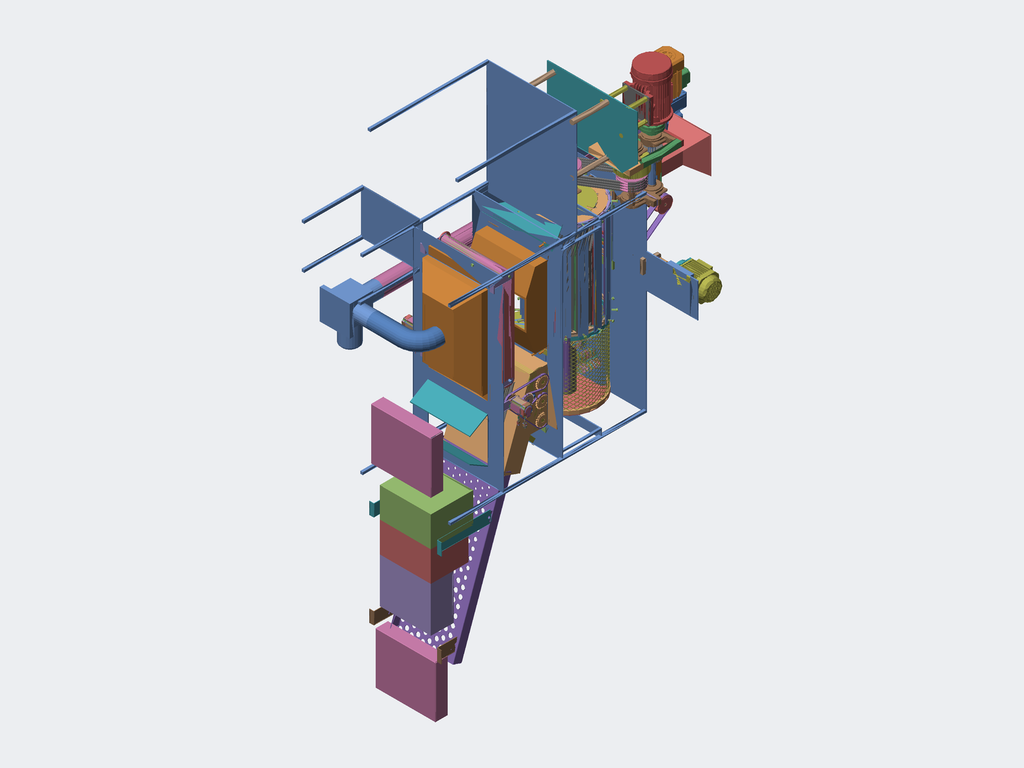Assembly | SolidWorks | 108 different items | 293 placed
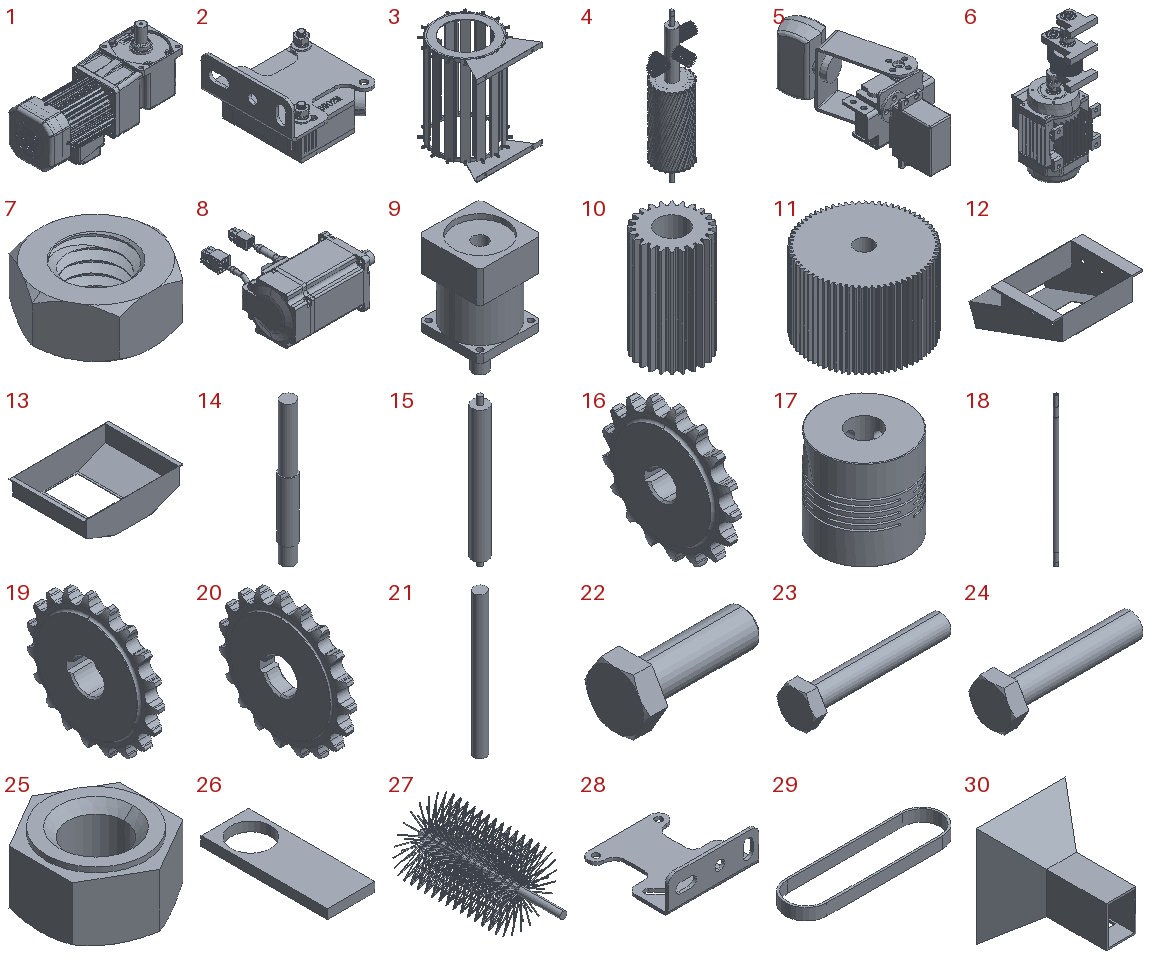Parts list (item | name | quantity | parent item | size | volume | features):
1 | (subassembly) | x1 | - | - | 5746372 mm3 | -
2 | (subassembly) | x1 | - | 60 x 58 x 40 mm | 49039 mm3 | features CompositeCurve 4
3 | (subassembly) | x1 | - | 488.345 x 547.074 x 650 mm | 5070939 mm3 | features ReferencePattern 72, LocalCirPattern 2, MirrorCompFeat 1
4 | (subassembly) | x1 | - | - | 9398103 mm3 | features ReferencePattern 46, LocalCirPattern 2
5 | (subassembly) | x1 | - | 62.179 x 144.352 x 61.763 mm | 114357 mm3 | features MirrorCompFeat 1
6 | (subassembly) | x1 | - | 154 x 213.028 x 468.972 mm | 4044827 mm3 | features AEMSimFeature 1
7 | - | x2 | in 2 | 7.91 x 6.85 x 3.05 mm | 87.239 mm3 | features Chamfer 1, Extrusion 1, Helix 1, ICE 1, RevCut 1, SweepCut 1
8 | - | x2 | - | - | - | features RefSurface 10
9 | - | x1 | - | 60 x 60 x 113 mm | 251469 mm3 | features ICE 7, Extrusion 1, RefAxis 1, RevCut 1
10 | - | x1 | in 6 | 26 x 26 x 44 mm | 14300 mm3 | features BaseBody 1, ICE 1
11 | - | x1 | in 6 | 71.959 x 72 x 50 mm | 185483 mm3 | features ICE 2, BaseBody 1
12 | - | x1 | - | 520 x 538.979 x 311.271 mm | 1451807 mm3 | features ICE 4, Extrusion 1, Shell 1
13 | - | x1 | - | 540 x 400 x 150 mm | 765108 mm3 | features ICE 3, Extrusion 1, Shell 1
14 | - | x1 | - | 40 x 40 x 355 mm | 385729 mm3 | features ICE 2, Extrusion 1
15 | - | x1 | - | 50 x 50 x 470 mm | 833504 mm3 | features ICE 2, Extrusion 1
16 | - | x2 | - | 15 x 73.539 x 73.841 mm | 33361 mm3 | features Chamfer 2, Cut 2, Revolution 2, CirPattern 1
17 | - | x2 | in 6 | 34 x 34 x 35 mm | 24409 mm3 | features BaseBody 1
18 | - | x2 | in 4 | 40 x 40 x 1400 mm | 1632189 mm3 | features ICE 6, Chamfer 4, 3DProfileFeature 1, Extrusion 1, HoleWzd 1, MoveCopyBody 1
19 | - | x3 | - | 15 x 81.595 x 81.862 mm | 41818 mm3 | features Chamfer 2, Cut 2, Revolution 2, CirPattern 1
20 | - | x1 | - | 9.37 x 81.595 x 81.862 mm | 34307 mm3 | features Chamfer 3, Cut 2, Revolution 2, CirPattern 1
21 | - | x1 | - | 30 x 30 x 352 mm | 248814 mm3 | features Extrusion 1, ICE 1
22 | - | x13 | - | 36.4 x 18.475 x 16 mm | 3737 mm3 | features BaseBody 1, Chamfer 1, ICE 1
23 | - | x48 | in 4 | 55.3 x 15.011 x 13 mm | 3267 mm3 | features BaseBody 1, MoveFace 1
24 | - | x30 | in 3 | 45.3 x 15.011 x 13 mm | 2757 mm3 | features BaseBody 1, RefAxis 1
25 | - | x1 | - | 13 x 15.011 x 7.5 mm | 785.095 mm3 | features BaseBody 1
26 | - | x1 | - | 60 x 160 x 12 mm | 91638 mm3 | features Extrusion 1, ICE 1
27 | - | x4 | in 4 | 100 x 200 x 100 mm | 28903 mm3 | features CirPattern 1, Extrusion 1, ICE 1, LPattern 1, RefAxis 1
28 | - | x1 | in 2 | 58 x 60 x 22 mm | 6510 mm3 | features ICE 3, MirrorPattern 2, SketchHole 2, EdgeFlange 1, Fillet 1, FlatPattern 1, SMBaseFlange 1, SheetMetal 1
29 | - | x1 | - | 378 x 100 x 28 mm | 119623 mm3 | features Extrusion 1
30 | - | x1 | - | 240 x 270 x 270 mm | 740709 mm3 | features ICE 3, Blend 1, Extrusion 1, Shell 1
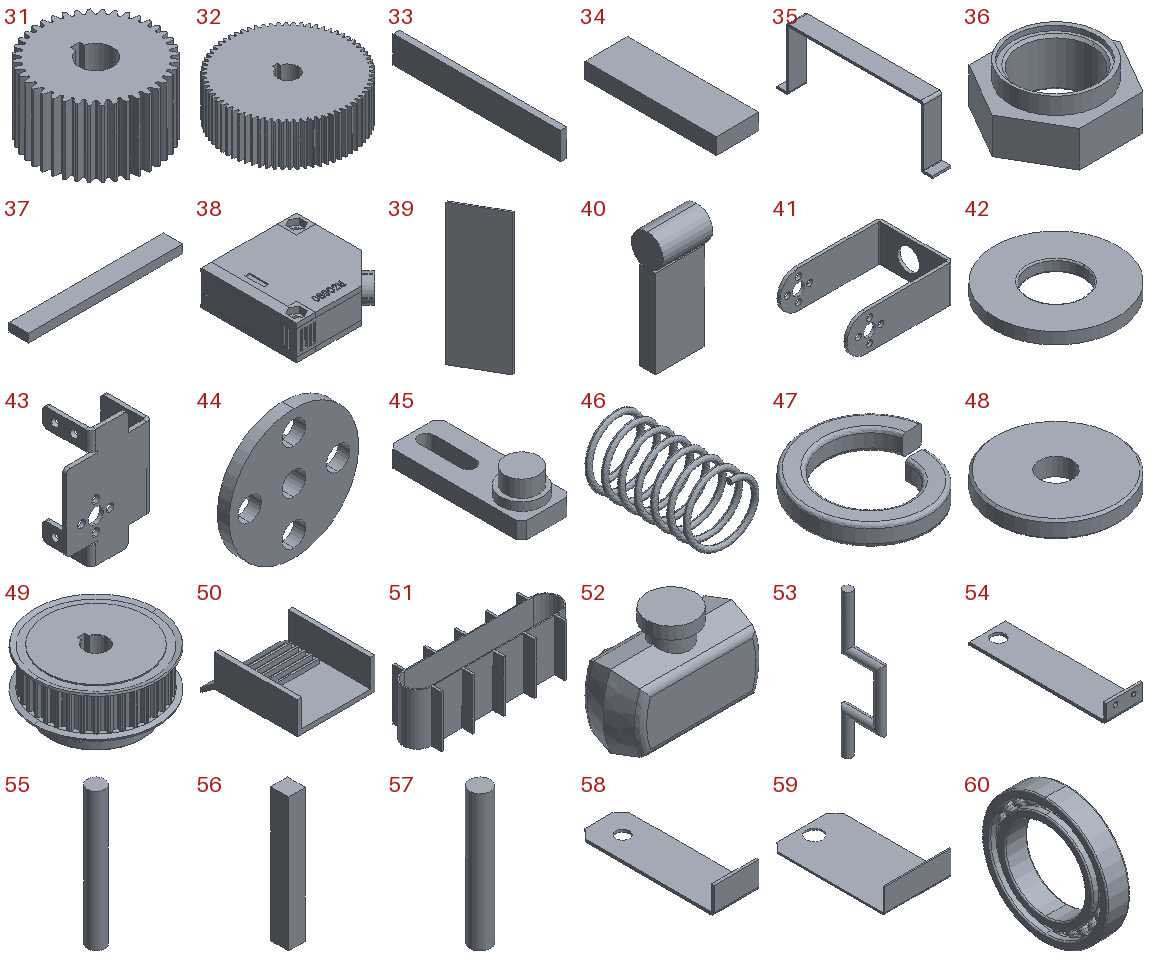31 | - | x1 | - | 104.808 x 104.808 x 60 mm | 422775 mm3 | features ICE 3, CirPattern 1, Extrusion 1, RefAxis 1
32 | - | x1 | - | 180 x 179.897 x 60 mm | 1397109 mm3 | features ICE 3, CirPattern 1, Extrusion 1, RefAxis 1
33 | - | x1 | - | 8 x 210 x 34 mm | 57120 mm3 | features Extrusion 1
34 | - | x1 | - | 90 x 275 x 34 mm | 841500 mm3 | features Extrusion 1
35 | - | x1 | - | 40 x 340 x 135 mm | 118889 mm3 | features EdgeFlange 2, FlatPattern 1, SMBaseFlange 1, SheetMetal 1
36 | - | x1 | - | 53.116 x 46 x 22 mm | 19269 mm3 | features ICE 3, Chamfer 1, Extrusion 1
37 | - | x1 | - | 275 x 34 x 15 mm | 140250 mm3 | features Extrusion 1
38 | - | x1 | in 2 | 50 x 50 x 18 mm | 41624 mm3 | features ICE 29, LPattern 4, CirPattern 2, Fillet 2, Chamfer 1, Extrusion 1, MirrorPattern 1
39 | - | x2 | - | 74.282 x 120 x 400 mm | 240000 mm3 | features Extrusion 1
40 | - | x1 | - | 62 x 50 x 150 mm | 220595 mm3 | features ICE 2, Extrusion 1
41 | - | x1 | in 5 | 71.712 x 49.895 x 25 mm | 8226 mm3 | features ICE 3, FlatPattern 1, SM3dBend 1, SMBaseFlange 1, SheetMetal 1
42 | - | x2 | in 2 | 9.05 x 9.05 x 0.85 mm | 43.941 mm3 | features Extrusion 1, Fillet 1, ICE 1
43 | - | x1 | in 5 | 45 x 25 x 62 mm | 6846 mm3 | features ICE 5, Fillet 3, EdgeFlange 2, SMBaseFlange 2, FlatPattern 1, MirrorPattern 1, SheetMetal 1
44 | - | x2 | in 5 | 22 x 6 x 22 mm | 838.805 mm3 | features ICE 2, Extrusion 1
45 | - | x1 | - | 30 x 80 x 25 mm | 26530 mm3 | features ICE 3, Chamfer 1, Extrusion 1
46 | - | x30 | in 3 | 12 x 23.5 x 12 mm | 203.726 mm3 | features Helix 1, Sweep 1
47 | - | x2 | in 2 | 6.6 x 6.6 x 2.189 mm | 20.119 mm3 | features Helix 1, Sweep 1
48 | - | x1 | - | 56 x 56 x 8 mm | 18117 mm3 | features Chamfer 1, Extrusion 1
49 | - | x2 | - | 99 x 99 x 48.077 mm | 252335 mm3 | features BaseBody 1
50 | - | x1 | - | 170 x 210 x 91.006 mm | 600000 mm3 | features ICE 3, Extrusion 1, LPattern 1
51 | - | x1 | - | 304 x 94 x 100 mm | 212673 mm3 | features ICE 2, LPattern 2, Extrusion 1
52 | - | x1 | in 5 | - | - | features ICE 4, Fillet 3, Extrusion 1, RevolvRefSurf 1
53 | - | x1 | - | 14 x 64 x 220 mm | 49260 mm3 | features Sweep 1
54 | - | x4 | - | 40 x 150 x 20 mm | 19277 mm3 | features ICE 2, EdgeFlange 1, FlatPattern 1, SMBaseFlange 1, SheetMetal 1
55 | - | x4 | - | 30 x 30 x 236 mm | 166819 mm3 | features Extrusion 1
56 | - | x2 | - | 32 x 34 x 253 mm | 275264 mm3 | features Extrusion 1
57 | - | x4 | - | 25 x 25 x 165 mm | 80994 mm3 | features Extrusion 1
58 | - | x5 | - | 50 x 154 x 30 mm | 26176 mm3 | features Chamfer 1, EdgeFlange 1, FlatPattern 1, ICE 1, SMBaseFlange 1, SheetMetal 1
59 | - | x2 | - | 80 x 140 x 30 mm | 25932 mm3 | features Chamfer 1, EdgeFlange 1, FlatPattern 1, ICE 1, SMBaseFlange 1, SheetMetal 1
60 | - | x2 | - | 10 x 55 x 55 mm | 10471 mm3 | features BaseBody 25
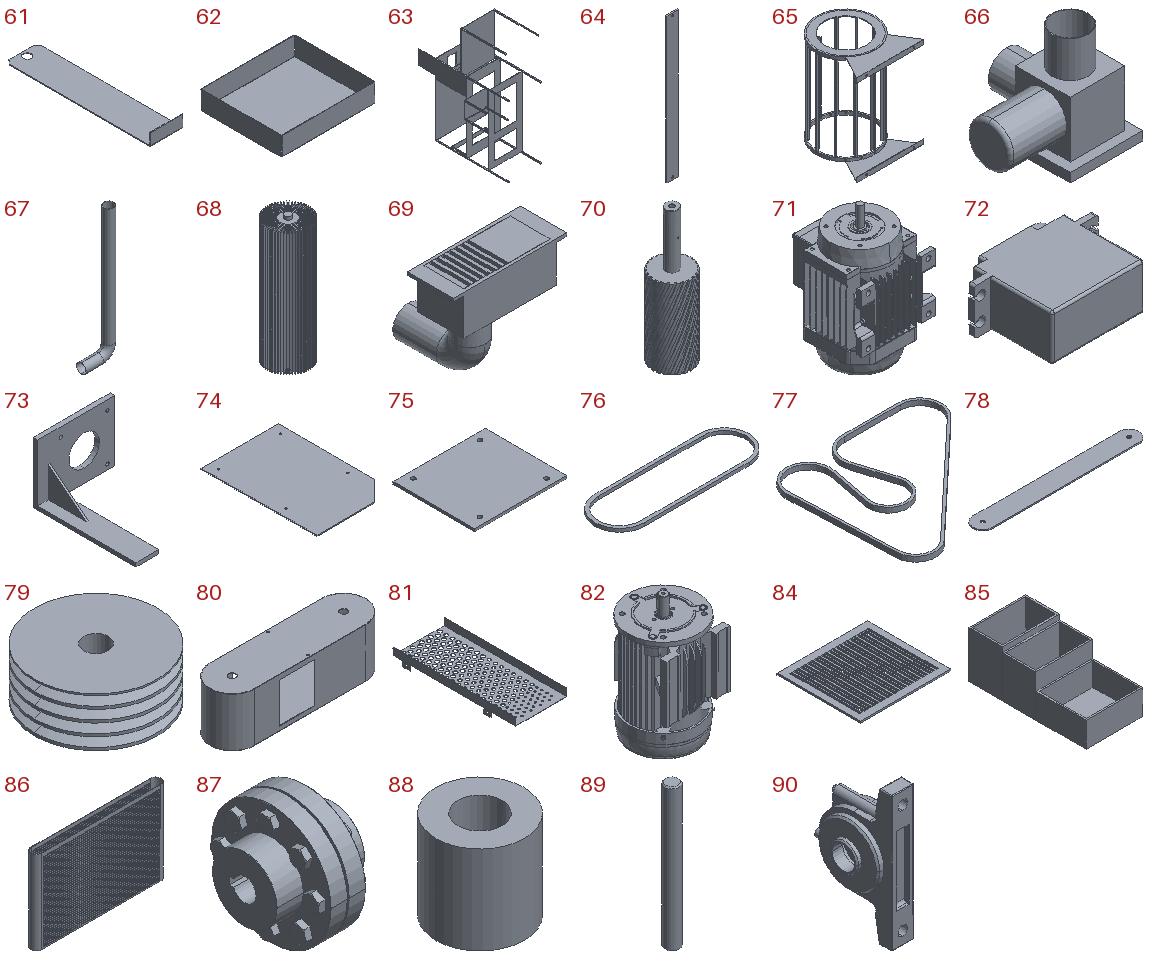61 | - | x2 | - | 80 x 360 x 30 mm | 61132 mm3 | features Chamfer 1, EdgeFlange 1, FlatPattern 1, ICE 1, SMBaseFlange 1, SheetMetal 1
62 | - | x2 | - | 400 x 345 x 80 mm | 502813 mm3 | features EdgeFlange 1, FlatPattern 1, SMBaseFlange 1, SheetMetal 1
63 | - | x1 | - | 1333 x 1609 x 1972 mm | 16595563 mm3 | features ICE 26, MirrorPattern 3, Cut 1, Extrusion 1, LPattern 1
64 | - | x15 | in 3 | 50 x 5 x 650 mm | 161997 mm3 | features Extrusion 1, ICE 1
65 | - | x1 | in 3 | 479.111 x 529 x 650 mm | 2552099 mm3 | features ICE 8, CirPattern 2, MirrorSolid 2, Extrusion 1
66 | - | x1 | - | 329 x 275 x 279 mm | 6409711 mm3 | features ICE 5, Extrusion 1, Fillet 1
67 | - | x1 | - | 325 x 100 x 1340 mm | 1391490 mm3 | features Shell 1, Sweep 1
68 | - | x3 | - | 128 x 128 x 425 mm | 2538969 mm3 | features ICE 3, CirPattern 1, Extrusion 1
69 | - | x1 | - | 370 x 275 x 315 mm | 2000718 mm3 | features ICE 6, Shell 2, Chamfer 1, Extrusion 1, LPattern 1, Sweep 1
70 | - | x1 | in 4 | 320.001 x 320.001 x 1100 mm | 7493467 mm3 | features ICE 12, CirPattern 1, Extrusion 1, Helix 1, Sweep 1
71 | - | x1 | in 6 | 154 x 190 x 270 mm | 3515361 mm3 | features BaseBody 2, ICE 1
72 | - | x2 | in 5 | 54 x 43 x 20 mm | 30390 mm3 | features ICE 5, 3DProfileFeature 1, Extrusion 1, Fillet 1, HoleWzd 1
73 | - | x1 | - | 202 x 270 x 160 mm | 499598 mm3 | features ICE 2, Extrusion 1, Gusset 1, HoleWzd 1
74 | - | x1 | - | 400 x 600 x 5 mm | 1173728 mm3 | features Chamfer 1, Extrusion 1, ICE 1
75 | - | x1 | - | 180 x 160 x 5 mm | 142995 mm3 | features Extrusion 1, ICE 1
76 | - | x4 | - | 470 x 150 x 10 mm | 107982 mm3 | features Extrusion 1
77 | - | x1 | - | 307.239 x 291.218 x 10 mm | 65563 mm3 | features BeltProfileFeature 1, ExtruThin 1
78 | - | x2 | - | 680 x 80 x 5 mm | 263366 mm3 | features Extrusion 1, ICE 1
79 | - | x2 | - | 150 x 150 x 60 mm | 903652 mm3 | features Extrusion 1, RevCut 1
80 | - | x1 | - | 350 x 100 x 111 mm | 133465 mm3 | features ICE 5, Extrusion 1, Shell 1
81 | - | x1 | - | 420 x 1000 x 100 mm | 925367 mm3 | features ICE 8, LPattern 6, EdgeFlange 1, Fillet 1, FlatPattern 1, MirrorPattern 1, SMBaseFlange 1, SheetMetal 1
82 | - | x1 | - | 200 x 200 x 344.5 mm | 7028641 mm3 | features ICE 8, BaseBody 1
83 | - | x1 | - | - | - | -
84 | - | x1 | - | 260 x 240 x 5 mm | 174000 mm3 | features Extrusion 1, ICE 1, LPattern 1
85 | - | x1 | - | 340 x 700 x 280 mm | 9420000 mm3 | features Shell 3, ICE 2, Extrusion 1
86 | - | x1 | - | - | 959871 mm3 | features LPattern 2, Extrusion 1, ICE 1
87 | - | x1 | - | 92 x 125 x 125 mm | 604795 mm3 | features ICE 4, Chamfer 2, BaseBody 1, Scale 1
88 | - | x2 | - | 60 x 60 x 60 mm | 143822 mm3 | features ICE 2, Extrusion 1
89 | - | x3 | in 6 | 12 x 12 x 120 mm | 13536 mm3 | features Chamfer 1, Extrusion 1
90 | - | x6 | - | 66 x 114 x 210 mm | 426890 mm3 | features BaseBody 1
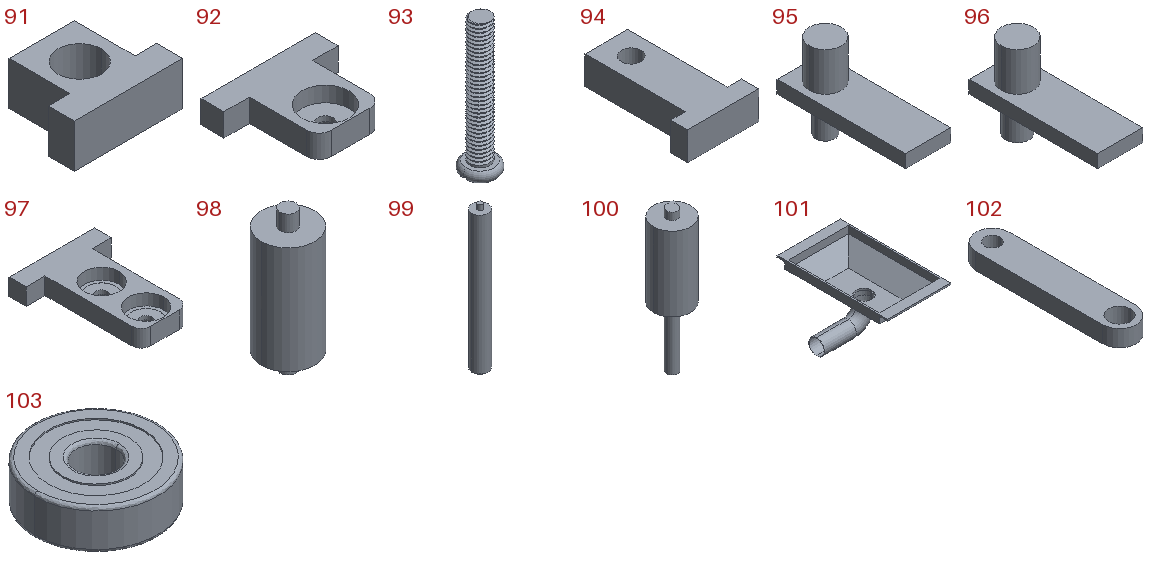91 | - | x1 | - | 50 x 40 x 20 mm | 22517 mm3 | features ICE 2, Extrusion 1
92 | - | x2 | in 6 | 90 x 73 x 18 mm | 63964 mm3 | features ICE 5, Fillet 4, Extrusion 1, LPattern 1
93 | - | x2 | in 2 | 6.8 x 6.8 x 27.2 mm | 311.216 mm3 | features ICE 4, Chamfer 1, Extrusion 1, Fillet 1, Helix 1, RevCut 1, Revolution 1, SweepCut 1
94 | - | x1 | - | 50 x 82.5 x 20 mm | 51221 mm3 | features ICE 2, Extrusion 1
95 | - | x1 | - | 35 x 100 x 65 mm | 54144 mm3 | features ICE 2, Extrusion 1
96 | - | x1 | - | 35 x 100 x 65 mm | 56088 mm3 | features ICE 2, Extrusion 1
97 | - | x1 | in 6 | 90 x 120 x 18 mm | 92684 mm3 | features ICE 4, Fillet 3, Extrusion 1, LPattern 1
98 | - | x1 | - | 50 x 50 x 130 mm | 201651 mm3 | features ICE 2, Extrusion 1
99 | - | x1 | - | 50 x 50 x 450 mm | 829970 mm3 | features ICE 2, Extrusion 1
100 | - | x1 | - | 50 x 50 x 190 mm | 212254 mm3 | features ICE 2, Extrusion 1
101 | - | x1 | - | 500 x 700 x 325 mm | 4429815 mm3 | features ICE 4, Shell 2, Chamfer 1, Extrusion 1, Sweep 1
102 | - | x1 | - | 30 x 145 x 15 mm | 55331 mm3 | features Extrusion 1, ICE 1
103 | - | x4 | in 6 | 37 x 37 x 12 mm | 8313 mm3 | features BaseBody 1
104 | DJ-750W.stp | x1 | - | - | - | -
105 | FCGZH-145.stp | x1 | - | - | - | -
106 | JXH-1.stp | x1 | - | - | - | -
107 | ZJZSJSX-750W.stp | x1 | - | - | - | -
108 | s750rt-U.stp (subassembly) | x1 | - | - | - | -
Mates (type | each side: item.copy, entity, surface, feature):
In the top assembly
Concentric | 48.1 face cylinder Boss-Extrude 1 | 22.1 face cylinder 输入1
Coincident | 48.1 face plane Boss-Extrude 1 | 22.1 face plane 输入1
Coincident | 48.1 face plane Boss-Extrude 1 | 18.1 face plane Boss-Extrude 1
Concentric | 18.1 face cylinder Boss-Extrude 2 | 90.1 face cylinder 输入1
Parallel | 90.1 face plane 输入1 | assembly plane
DistanceDim | 90.1 face plane 输入1 | 18.1 face plane Boss-Extrude 3
Coincident | 90.1 face plane 输入1 | 90.2 face plane 输入1
Concentric | 18.1 face cylinder Boss-Extrude 3 | 90.2 face cylinder 输入1
DistanceDim | 90.2 face plane 输入1 | 18.1 face plane Boss-Extrude 6
Coincident | 18.1 face plane Boss-Extrude 6 | 18.2 face plane Boss-Extrude 6
Concentric | 18.1 face cylinder Boss-Extrude 3 | 18.2 face cylinder Boss-Extrude 4
Parallel | 63.1 face plane Boss-Extrude 2 | assembly plane
Coincident | 63.1 plane | assembly plane
Coincident | 63.1 face plane Boss-Extrude 2 | 25.1 face plane 输入1
DistanceDim | 30.1 plane | 63.1 face plane Boss-Extrude 1
Coincident | 30.1 plane | assembly plane
Coincident | 90.2 face plane 输入1 | 36.1 face plane Boss-Extrude 1
Concentric | 18.2 face cylinder Boss-Extrude 6 | 36.1 face cylinder Cut-Extrude 2
Coincident | 90.2 plane | 60.1 plane
Concentric | 18.2 face cylinder Boss-Extrude 6 | 60.1 face cylinder 输入23
Concentric | 48.1 face cylinder Boss-Extrude 1 | 60.2 face cylinder 输入8
Coincident | 90.1 plane | 60.2 plane
Concentric | 70.1 face cylinder Boss-Extrude 4 | 83.1 face cylinder Boss-Extrude 2
Coincident | 83.1 face plane Boss-Extrude 2 | 65.1 face plane Mirror 7
Coincident | 90.1 face plane 输入1 | 22.2 face plane 输入1
Concentric | 90.1 face cylinder 输入1 | 22.2 face cylinder 输入1
Coincident | 90.1 face plane 输入1 | 22.3 face plane 输入1
Concentric | 90.1 face cylinder 输入1 | 22.3 face cylinder 输入1
Coincident | 90.2 face plane 输入1 | 22.4 face plane 输入1
Concentric | 90.2 face cylinder 输入1 | 22.4 face cylinder 输入1
Coincident | 90.2 face plane 输入1 | 22.5 face plane 输入1
Concentric | 90.2 face cylinder 输入1 | 22.5 face cylinder 输入1
Coincident | 65.1 face plane Mirror 10 | 22.6 face plane 输入1
Concentric | 65.1 face cylinder Mirror 10 | 22.6 face cylinder 输入1
Coincident | 65.1 face plane Mirror 10 | 22.7 face plane 输入1
Concentric | 65.1 face cylinder Mirror 10 | 22.7 face cylinder 输入1
Coincident | 65.1 face plane Boss-Extrude 5 | 22.8 face plane 输入1
Concentric | 65.1 face cylinder Cut-Extrude 3 | 22.8 face cylinder 输入1
Coincident | 83.1 face plane Boss-Extrude 4 | 22.9 face plane 输入1
Concentric | 83.1 face cylinder Cut-Extrude 1 | 22.9 face cylinder 输入1
Coincident | 83.1 face plane Boss-Extrude 4 | 22.10 face plane 输入1
Concentric | 83.1 face cylinder Cut-Extrude 1 | 22.10 face cylinder 输入1
Coincident | 65.1 face plane Boss-Extrude 5 | 22.11 face plane 输入1
Concentric | 65.1 face cylinder Cut-Extrude 3 | 22.11 face cylinder 输入1
Coincident | 83.1 face plane Mirror 5 | 22.12 face plane 输入1
Concentric | 83.1 face cylinder Mirror 5 | 22.12 face cylinder 输入1
Coincident | 83.1 face plane Mirror 5 | 22.13 face plane 输入1
Concentric | 83.1 face cylinder Mirror 5 | 22.13 face cylinder 输入1
DistanceDim | 90.2 face plane 输入1 | 63.1 face plane Boss-Extrude 1
Coincident | 90.1 face plane 输入1 | 63.1 face plane Boss-Extrude 6
Coincident | 90.1 face plane 输入1 | 63.1 face plane Boss-Extrude 1
Concentric | 70.1 face cylinder Boss-Extrude 8 | 65.1 face cylinder Boss-Extrude 6
Coincident | 63.1 face plane Boss-Extrude 1 | 90.3 face plane 输入1
Coincident | 90.3 face plane 输入1 | 33.1 face plane Boss-Extrude 1 | 3 times
Coincident | 63.1 face plane Boss-Extrude 8 | 33.1 face plane Boss-Extrude 1
Concentric | 100.1 face cylinder Boss-Extrude 1 | 51.1 face cylinder Boss-Extrude 1
Coincident | 100.1 face plane Boss-Extrude 1 | 51.1 face plane Boss-Extrude 1
Concentric | 51.1 face cylinder Boss-Extrude 1 | 80.1 face cylinder Boss-Extrude 1 | 2 times
Width | 80.1 face plane Boss-Extrude 1 | 80.1 face plane Boss-Extrude 2 | 51.1 face plane Boss-Extrude 1 | 51.1 face plane Boss-Extrude 1
Concentric | 51.1 face cylinder Boss-Extrude 1 | 98.1 face cylinder Boss-Extrude 1
Coincident | 51.1 face plane Boss-Extrude 1 | 98.1 face plane Boss-Extrude 1
Coincident | 80.1 face plane Boss-Extrude 2 | 54.1 face plane Base-Flange 1
Concentric | 98.1 face cylinder Boss-Extrude 2 | 54.1 face cylinder Cut-Extrude 1
Concentric | 98.1 face cylinder Boss-Extrude 3 | 54.2 face cylinder Cut-Extrude 1
Coincident | 80.1 face plane Boss-Extrude 1 | 54.2 face plane Base-Flange 1
Coincident | 80.1 face plane Boss-Extrude 2 | 54.3 face plane Base-Flange 1
Concentric | 100.1 face cylinder Boss-Extrude 3 | 54.3 face cylinder Cut-Extrude 1
Coincident | 80.1 face plane Boss-Extrude 1 | 54.4 face plane Base-Flange 1
Concentric | 100.1 face cylinder Boss-Extrude 2 | 54.4 face cylinder Cut-Extrude 1
DistanceDim | 54.1 face plane Edge-Flange 1 | 63.1 face plane Boss-Extrude 1
Coincident | 90.3 face plane 输入1 | 21.1 face plane Boss-Extrude 1
Concentric | 21.1 face cylinder Boss-Extrude 1 | 90.4 face cylinder 输入1
Coincident | 54.1 face plane Edge-Flange 1 | 54.2 face plane Edge-Flange 1
Coincident | 54.1 face plane Edge-Flange 1 | 54.3 face plane Edge-Flange 1
Coincident | 54.4 face plane Edge-Flange 1 | 54.3 face plane Edge-Flange 1
Coincident | 63.1 face plane Boss-Extrude 1 | 90.5 face plane 输入1
Coincident | 31.1 face plane Boss-Extrude 1 | 32.1 face plane Boss-Extrude 1
DistanceDim | 31.1 face plane Boss-Extrude 1 | 90.4 face plane 输入1
Coincident | 90.4 face plane 输入1 | 74.1 face plane Boss-Extrude 1
Parallel | 90.4 face plane 输入1 | 74.1 face plane Boss-Extrude 1
Coincident | 74.1 face plane Boss-Extrude 1 | 34.1 face plane Boss-Extrude 1
Coincident | 90.4 face plane 输入1 | 34.1 face plane Boss-Extrude 1
Concentric | 90.6 face cylinder 输入1 | 14.1 face cylinder Boss-Extrude 2
Coincident | 32.1 face plane Boss-Extrude 1 | 14.1 face plane Boss-Extrude 1
Concentric | 90.5 face cylinder 输入1 | 14.1 face cylinder Boss-Extrude 3
Coincident | 90.5 face plane 输入1 | 14.1 face plane Boss-Extrude 1
Parallel | 90.6 face plane 输入1 | 74.1 face plane Boss-Extrude 1
Coincident | 63.1 face plane Boss-Extrude 1 | 85.1 face plane Boss-Extrude 1 | 2 times
Concentric | 74.1 face cylinder Cut-Extrude 1 | 55.1 face cylinder Boss-Extrude 1
Coincident | 74.1 face plane Boss-Extrude 1 | 55.1 face plane Boss-Extrude 1
Concentric | 74.1 face cylinder Cut-Extrude 1 | 55.2 face cylinder Boss-Extrude 1
Coincident | 74.1 face plane Boss-Extrude 1 | 55.2 face plane Boss-Extrude 1
Coincident | 74.1 face plane Boss-Extrude 1 | 55.3 face plane Boss-Extrude 1
Concentric | 74.1 face cylinder Cut-Extrude 1 | 55.3 face cylinder Boss-Extrude 1
Concentric | 74.1 face cylinder Cut-Extrude 1 | 55.4 face cylinder Boss-Extrude 1
Coincident | 74.1 face plane Boss-Extrude 1 | 55.4 face plane Boss-Extrude 1
Concentric | 87.1 face cylinder Cut-Extrude 2 | 82.1 face cylinder 输入1
Parallel | 63.1 face plane Boss-Extrude 11 | 55.2 face plane Boss-Extrude 1
Coincident | 34.1 face plane Boss-Extrude 1 | 56.1 face plane Boss-Extrude 1 | 3 times
Coincident | 90.4 face plane 输入1 | 90.6 face plane 输入1
Parallel | 82.1 face plane Boss-Extrude 2 | 74.1 face plane Boss-Extrude 1
DistanceDim | 87.1 face plane Boss-Extrude 1 | 82.1 face plane 输入1
Coincident | 81.1 face plane Boss-Extrude 1 | 59.1 face plane Base-Flange 1
Concentric | 81.1 face cylinder Cut-Extrude 7 | 59.1 face cylinder Cut-Extrude 1
Coincident | 63.1 face plane Boss-Extrude 1 | 59.1 face plane Edge-Flange 1
Width | 63.1 face plane Boss-Extrude 1 | 63.1 face plane Boss-Extrude 1 | 81.1 face plane Edge-Flange 1 | 81.1 face plane Edge-Flange 1
Width | 81.1 face plane Edge-Flange 1 | 81.1 face plane Edge-Flange 1 | 85.1 face plane Boss-Extrude 1 | 85.1 face plane Boss-Extrude 1
DistanceDim | 63.1 face plane Boss-Extrude 1 | 59.1 face plane Base-Flange 1
Coincident | 59.1 face plane Edge-Flange 1 | 59.2 face plane Edge-Flange 1
Concentric | 81.1 face cylinder Cut-Extrude 7 | 59.2 face cylinder Cut-Extrude 1
Coincident | 81.1 face plane Mirror 1 | 59.2 face plane Base-Flange 1
Coincident | 59.2 face plane Edge-Flange 1 | 62.1 face plane Base-Flange 1
DistanceDim | 59.2 face plane Edge-Flange 1 | 62.1 face plane Edge-Flange 1
Coincident | 82.1 face plane Boss-Extrude 2 | 75.1 face plane Boss-Extrude 1
Coincident | 82.1 face plane 输入1 | 75.1 face plane Boss-Extrude 1 | 2 times
Coincident | 75.1 face plane Boss-Extrude 1 | 57.1 face plane Boss-Extrude 1
Concentric | 75.1 face cylinder Cut-Extrude 1 | 57.1 face cylinder Boss-Extrude 1
Concentric | 75.1 face cylinder Cut-Extrude 1 | 57.2 face cylinder Boss-Extrude 1
Coincident | 75.1 face plane Boss-Extrude 1 | 57.2 face plane Boss-Extrude 1
Concentric | 75.1 face cylinder Cut-Extrude 1 | 57.3 face cylinder Boss-Extrude 1
Coincident | 75.1 face plane Boss-Extrude 1 | 57.3 face plane Boss-Extrude 1
Concentric | 75.1 face cylinder Cut-Extrude 1 | 57.4 face cylinder Boss-Extrude 1
Coincident | 75.1 face plane Boss-Extrude 1 | 57.4 face plane Boss-Extrude 1
Coincident | 81.1 face plane Boss-Extrude 1 | 61.1 face plane Base-Flange 1
Concentric | 81.1 face cylinder Cut-Extrude 7 | 61.1 face cylinder Cut-Extrude 1
Parallel | 59.1 face plane Edge-Flange 1 | 61.1 face plane Edge-Flange 1
Coincident | 85.1 face plane Boss-Extrude 2 | 61.1 face plane Edge-Flange 1
Coincident | 81.1 face plane Mirror 1 | 61.2 face plane Base-Flange 1
Concentric | 81.1 face cylinder Cut-Extrude 7 | 61.2 face cylinder Cut-Extrude 1
Coincident | 61.1 face plane Edge-Flange 1 | 61.2 face plane Edge-Flange 1
Coincident | 63.1 face plane Cut-Extrude 5 | 101.1 face plane Boss-Extrude 1 | 2 times
Coincident | 63.1 face plane Boss-Extrude 5 | 12.1 face plane Boss-Extrude 2
Coincident | 63.1 face plane Cut-Extrude 4 | 12.1 face plane Boss-Extrude 1 | 2 times
Coincident | 70.1 face plane Boss-Extrude 8 | 65.1 face plane Boss-Extrude 6
Parallel | 63.1 face plane Boss-Extrude 5 | 65.1 face plane Mirror 10
Coincident | 83.1 face plane Boss-Extrude 3 | 65.1 face plane Boss-Extrude 4
DistanceDim | 86.1 face plane Boss-Extrude 1 | 63.1 face plane Boss-Extrude 2
Coincident | 101.1 face plane Sweep 1 | 66.1 face plane Boss-Extrude 5
Parallel | 63.1 face plane Boss-Extrude 1 | 66.1 face plane Boss-Extrude 1
Concentric | 48.1 face cylinder Boss-Extrude 1 | 18.1 face cylinder M8 Tapped Hole 2
Coincident | 63.1 face plane Boss-Extrude 1 | 69.1 face plane Boss-Extrude 1
Width | 69.1 face plane Boss-Extrude 1 | 69.1 face plane Boss-Extrude 1 | 63.1 face plane Cut-Extrude 6 | 63.1 face plane Cut-Extrude 6
Coincident | 66.1 face plane Boss-Extrude 4 | 67.1 face plane Sweep 1
Concentric | 66.1 face cylinder Boss-Extrude 4 | 67.1 face cylinder Sweep 1
Concentric | 69.1 face cylinder Sweep 1 | 67.1 face cylinder Sweep 1
Coincident | 63.1 face plane Boss-Extrude 2 | 101.1 face plane Boss-Extrude 3
Width | 81.1 face plane Edge-Flange 1 | 81.1 face plane Edge-Flange 1 | 62.1 face plane Edge-Flange 1 | 62.1 face plane Edge-Flange 1
Coincident | 85.1 face plane Boss-Extrude 1 | 62.2 face plane Base-Flange 1
Coincident | 85.1 face plane Boss-Extrude 1 | 62.2 face plane Edge-Flange 1
Coincident | 63.1 face plane Cut-Extrude 6 | 69.1 face plane LPattern 1
Coincident | 12.1 face plane Boss-Extrude 5 | 84.1 face plane Boss-Extrude 1
DistanceDim | 84.1 face plane Boss-Extrude 1 | 12.1 edge
DistanceDim | 84.1 face plane Boss-Extrude 1 | 12.1 face plane Cut-Extrude 1
Concentric | 12.1 face cylinder Cut-Extrude 2 | 68.1 face cylinder Boss-Extrude 3
Coincident | 12.1 face plane Boss-Extrude 1 | 68.1 face plane Boss-Extrude 2
Coincident | 63.1 face plane Boss-Extrude 2 | 39.1 face plane Boss-Extrude 1
Coincident | 63.1 face plane Boss-Extrude 2 | 39.2 face plane Boss-Extrude 1
Coincident | 63.1 face plane Cut-Extrude 7 | 39.1 face plane Boss-Extrude 1
Coincident | 63.1 face plane Cut-Extrude 7 | 39.1 edge
Coincident | 63.1 face plane Cut-Extrude 7 | 39.2 face plane Boss-Extrude 1
Coincident | 63.1 edge | 39.2 edge
Concentric | 68.1 face cylinder Boss-Extrude 3 | 19.1 face cylinder Revolve 1
Coincident | 68.1 face plane Boss-Extrude 3 | 19.1 face plane Revolve 1
Concentric | 86.1 face cylinder Boss-Extrude 1 | 15.1 face cylinder Boss-Extrude 1
Coincident | 86.1 face plane Boss-Extrude 1 | 15.1 face plane Boss-Extrude 1
Concentric | 86.1 face cylinder Boss-Extrude 1 | 99.1 face cylinder Boss-Extrude 1
Coincident | 86.1 face plane Boss-Extrude 1 | 99.1 face plane Boss-Extrude 1
Concentric | 15.1 face cylinder Boss-Extrude 3 | 16.1 face cylinder Revolve 1
Coincident | 15.1 face plane Boss-Extrude 3 | 16.1 face plane Revolve 1
Coincident | 99.1 face plane Boss-Extrude 1 | 78.1 face plane Boss-Extrude 1
Concentric | 99.1 face cylinder Boss-Extrude 2 | 78.1 face cylinder Cut-Extrude 1
Concentric | 15.1 face cylinder Boss-Extrude 3 | 78.1 face cylinder Cut-Extrude 1
Coincident | 19.1 face plane Revolve 1 | 16.1 face plane Revolve 1
Coincident | 15.1 face plane Boss-Extrude 1 | 78.2 face plane Boss-Extrude 1
Concentric | 15.1 face cylinder Boss-Extrude 2 | 78.2 face cylinder Cut-Extrude 1
Concentric | 99.1 face cylinder Boss-Extrude 3 | 78.2 face cylinder Cut-Extrude 1
Coincident | 78.2 face plane Boss-Extrude 1 | 58.1 face plane Base-Flange 1
Concentric | 99.1 face cylinder Boss-Extrude 3 | 58.1 face cylinder Cut-Extrude 1
Parallel | 63.1 face plane Boss-Extrude 2 | 58.1 face plane Edge-Flange 1
Coincident | 78.1 face plane Boss-Extrude 1 | 58.2 face plane Base-Flange 1
Concentric | 99.1 face cylinder Boss-Extrude 2 | 58.2 face cylinder Cut-Extrude 1
Parallel | 63.1 face plane Boss-Extrude 2 | 58.2 face plane Edge-Flange 1
Concentric | 15.1 face cylinder Boss-Extrude 2 | 58.3 face cylinder Cut-Extrude 1
Coincident | 78.2 face plane Boss-Extrude 1 | 58.3 face plane Base-Flange 1
Parallel | 63.1 face plane Boss-Extrude 2 | 58.3 face plane Edge-Flange 1
Coincident | 78.1 face plane Boss-Extrude 1 | 58.4 face plane Base-Flange 1
Concentric | 15.1 face cylinder Boss-Extrude 3 | 58.4 face cylinder Cut-Extrude 1
Parallel | 63.1 face plane Boss-Extrude 2 | 58.4 face plane Edge-Flange 1
Coincident | 54.3 face plane Edge-Flange 1 | 69.1 face plane Boss-Extrude 1
Coincident | 12.1 face plane Boss-Extrude 1 | 45.1 face plane Boss-Extrude 1
Concentric | 20.1 face cylinder Revolve 1 | 45.1 face cylinder Cut-Extrude 1
Coincident | 20.1 face plane Revolve 1 | 45.1 face plane Boss-Extrude 2
DistanceDim | 45.1 face plane Boss-Extrude 1 | 12.1 face plane Boss-Extrude 1
Coincident | 63.1 face plane Boss-Extrude 5 | 13.1 face plane Boss-Extrude 2
Coincident | 63.1 face plane Cut-Extrude 8 | 13.1 face plane Boss-Extrude 1
Coincident | 63.1 face plane LPattern 1 | 13.1 face plane Boss-Extrude 1
BeltDim | 19.1 edge | 20.1 edge
BeltDim | 20.1 edge | 19.2 edge
BeltDim | 19.2 edge | 19.3 edge
BeltDim | 16.1 edge | 19.1 edge
Concentric | 15.1 face cylinder Boss-Extrude 2 | 9.1 face cylinder Boss-Extrude 1
Concentric | 8.1 face cylinder 曲Face-输入1 | 9.1 face cylinder Cut-Extrude 3
Coincident | 8.1 face plane 曲Face-输入1 | 9.1 face plane Boss-Extrude 5 | 2 times
Concentric | 9.1 face cylinder Boss-Extrude 2 | 26.1 face cylinder Cut-Extrude 1
Coincident | 9.1 face plane Boss-Extrude 3 | 26.1 face plane Boss-Extrude 1
Parallel | 63.1 face plane Boss-Extrude 2 | 26.1 face plane Boss-Extrude 1
Coincident | 63.1 face plane Boss-Extrude 2 | 26.1 face plane Boss-Extrude 1
Concentric | 9.1 face cylinder Boss-Extrude 1 | 88.1 face cylinder Cut-Extrude 1
DistanceDim | 88.1 face plane Boss-Extrude 1 | 58.3 face plane Base-Flange 1
Coincident | 63.1 face plane Boss-Extrude 1 | 50.1 face plane Boss-Extrude 1
Coincident | 63.1 face plane Cut-Extrude 6 | 50.1 face plane Boss-Extrude 2
Coincident | 63.1 face plane Boss-Extrude 1 | 35.1 face plane Edge-Flange 2
Coincident | 54.2 face plane Edge-Flange 1 | 35.1 face plane Base-Flange 1
Width | 35.1 face plane Edge-Flange 1 | 35.1 face plane Edge-Flange 1 | 54.2 face plane Base-Flange 1 | 54.1 face plane Base-Flange 1
DistanceDim | 50.1 face plane Boss-Extrude 1 | 69.1 face plane Boss-Extrude 1
Coincident | 35.1 face plane Base-Flange 1 | 91.1 face plane Boss-Extrude 1
Coincident | 30.1 face plane Boss-Extrude 1 | 80.1 face plane Boss-Extrude 1
Coincident | 63.1 face plane Boss-Extrude 17 | 94.1 face plane Boss-Extrude 1
Concentric | 53.1 face cylinder Sweep 1 | 94.1 face cylinder Cut-Extrude 1
Coincident | 53.1 face plane Sweep 1 | 94.1 face plane Boss-Extrude 1
DistanceDim | 94.1 face plane Boss-Extrude 1 | 63.1 face plane Cut-Extrude 9
Coincident | 63.1 face plane Boss-Extrude 1 | 95.1 face plane Boss-Extrude 1
Coincident | 30.1 face plane Cut-Extrude 3 | 40.1 face plane Boss-Extrude 1 | 2 times
Concentric | 40.1 face cylinder Boss-Extrude 3 | 102.1 face cylinder Cut-Extrude 1
Coincident | 40.1 face plane Boss-Extrude 1 | 102.1 face plane Boss-Extrude 1
Concentric | 53.1 face cylinder Sweep 1 | 102.1 face cylinder Cut-Extrude 1
Coincident | 63.1 face plane Boss-Extrude 1 | 96.1 face plane Boss-Extrude 1
Coincident | 63.1 face plane Boss-Extrude 17 | 73.1 face plane Boss-Extrude 1 | 2 times
DistanceDim | 73.1 face plane Boss-Extrude 1 | 63.1 face plane Boss-Extrude 1
DistanceDim | 88.2 face plane Boss-Extrude 1 | 73.1 face plane Boss-Extrude 2
Coincident | 20.1 face plane Revolve 1 | 16.2 face plane Revolve 1
Concentric | 16.2 face cylinder Revolve 1 | 8.2 face cylinder 曲Face-输入1
Parallel | 63.1 face plane Boss-Extrude 2 | 8.2 face plane 曲Face-输入4
Coincident | 16.2 face plane Revolve 2 | 8.2 face plane 曲Face-输入1
Coincident | 8.2 face plane 曲Face-输入1 | 58.5 face plane Base-Flange 1
Concentric | 8.2 face cylinder 曲Face-输入1 | 58.5 face cylinder Cut-Extrude 1
Coincident | 37.1 face plane Boss-Extrude 1 | 56.2 face plane Boss-Extrude 1 | 3 times
Concentric | 87.1 face cylinder Cut-Extrude 2 | 14.1 face cylinder Boss-Extrude 2
Coincident | 87.1 face plane 输入1 | 90.6 face plane 输入1
Concentric | 21.1 face cylinder Boss-Extrude 1 | 32.1 face cylinder Cut-Extrude 2
Concentric | 31.1 face cylinder Cut-Extrude 2 | 14.1 face cylinder Boss-Extrude 2
Coincident | 90.3 face plane 输入1 | 90.5 face plane 输入1
Coincident | 34.1 face plane Boss-Extrude 1 | 56.2 face plane Boss-Extrude 1
Concentric | 90.3 face cylinder 输入1 | 21.1 face cylinder Boss-Extrude 1
Concentric | 21.1 face cylinder Boss-Extrude 1 | 79.1 face cylinder Boss-Extrude 1
Concentric | 18.2 face cylinder Boss-Extrude 1 | 79.2 face cylinder Boss-Extrude 1
Coincident | 79.1 face plane Boss-Extrude 1 | 79.2 face plane Boss-Extrude 1
Concentric | 79.2 face cylinder Boss-Extrude 1 | 76.1 face cylinder Boss-Extrude 1
Concentric | 21.1 face cylinder Boss-Extrude 1 | 76.1 face cylinder Boss-Extrude 1
Concentric | 100.1 face cylinder Boss-Extrude 2 | 49.1 face cylinder 输入1
DistanceDim | 49.1 face plane 输入1 | 100.1 face plane Boss-Extrude 1
Coincident | 63.1 face plane Boss-Extrude 1 | 97.1 face plane Boss-Extrude 1
Concentric | 92.1 face cylinder LPattern 1 | 49.2 face cylinder 输入1
Concentric | 49.2 face cylinder 输入1 | 89.1 face cylinder Boss-Extrude 1
Coincident | 17.1 face plane 输入1 | 89.1 face plane Boss-Extrude 1
Coincident | 49.2 face plane 输入1 | 89.1 face plane Boss-Extrude 1
Coincident | 49.1 face plane 输入1 | 49.2 face plane 输入1
Concentric | 89.1 face cylinder Boss-Extrude 1 | 29.1 face cylinder Boss-Extrude 1
Coincident | 49.2 face plane 输入1 | 29.1 face plane Boss-Extrude 1
Concentric | 100.1 face cylinder Boss-Extrude 3 | 29.1 face cylinder Boss-Extrude 1
Coincident | 63.1 face plane Boss-Extrude 5 | 43.1 face plane Base-Flange 1
Coincident | 63.1 face plane Boss-Extrude 1 | 43.1 face plane Mirror 1
Coincident | 61.2 face plane Base-Flange 1 | 28.1 face plane Edge-Flange 1
In subassembly 4
Concentric | 70.2 face cylinder Cut-Extrude 1 | 18.1 face cylinder Boss-Extrude 2
Coincident | 70.2 face plane Boss-Extrude 5 | 18.1 face plane Boss-Extrude 3
Concentric | 70.2 face cylinder Cut-Extrude 3 | 27.1 face cylinder Boss-Extrude 1
Concentric | 70.2 face cylinder Cut-Extrude 4 | 27.2 face cylinder Boss-Extrude 1
Concentric | 70.2 face cylinder Cut-Extrude 9 | 27.3 face cylinder Boss-Extrude 1
Concentric | 70.2 face cylinder Cut-Extrude 2 | 27.4 face cylinder Boss-Extrude 1
DistanceDim | 70.2 plane | 23.1 plane
DistanceDim | 23.1 plane | 70.2 face plane Boss-Extrude 8
Tangent | 70.2 face surface:4006 Sweep 1 | 23.1 face plane 输入1
Tangent | 70.2 face surface:4006 CirPattern 5 | 23.2 face plane 输入1
Parallel | 23.2 plane | 4.1 plane
Parallel | 4.1 plane | 23.2 plane
In subassembly 3
Coincident | 65.2 plane | 3.1 plane | 3 times
Concentric | 65.2 face cylinder CirPattern 1 | 64.1 face cylinder Cut-Extrude 1
Tangent | 65.2 face cylinder Boss-Extrude 1 | 64.1 face plane Boss-Extrude 1
Concentric | 64.1 face cylinder Cut-Extrude 1 | 24.1 face cylinder 输入1
Coincident | 24.1 axis | 46.1 select_type:24
In subassembly 6
Concentric | 71.1 face cylinder Cut-Extrude 1 | 10.1 face cylinder Boss-Extrude 1
Coincident | 10.1 plane | 11.1 plane
DistanceDim | 11.1 plane | 10.1 plane
Parallel | 71.1 face plane 输入1 | 10.1 plane
Coincident | 10.1 face plane 输入1 | 11.1 face plane 输入1
Concentric | 71.1 face cylinder Cut-Extrude 1 | 17.2 face cylinder 输入1
Coincident | 71.1 face plane 输入1 | 17.2 face plane 输入1
Concentric | 10.1 face cylinder Boss-Extrude 1 | 89.1 face cylinder Boss-Extrude 1
Coincident | 17.2 face plane 输入1 | 89.1 face plane Boss-Extrude 1
Concentric | 11.1 face cylinder Boss-Extrude 1 | 89.2 face cylinder Boss-Extrude 1
Concentric | 89.2 face cylinder Boss-Extrude 1 | 17.3 face cylinder 输入1
Coincident | 89.2 face plane Boss-Extrude 1 | 17.3 face plane 输入1
Concentric | 89.1 face cylinder Boss-Extrude 1 | 97.2 face cylinder Cut-Extrude 1
Parallel | 71.1 face plane 输入1 | 97.2 face plane Boss-Extrude 1
Coincident | 89.1 face plane Boss-Extrude 1 | 97.2 face plane Boss-Extrude 1
Concentric | 89.2 face cylinder Boss-Extrude 1 | 92.2 face cylinder LPattern 1
Coincident | 89.2 face plane Boss-Extrude 1 | 92.2 face plane Boss-Extrude 1
Parallel | 97.2 face plane Boss-Extrude 1 | 92.2 face plane Boss-Extrude 1
DistanceDim | 17.2 face plane 输入1 | 92.2 face plane Boss-Extrude 1
Concentric | 92.3 face cylinder LPattern 1 | 103.1 face cylinder 输入1
Coincident | 92.3 face plane Boss-Extrude 1 | 103.1 face plane 输入1
Coincident | 92.2 face plane Boss-Extrude 1 | 103.2 face plane 输入1
Concentric | 89.1 face cylinder Boss-Extrude 1 | 103.3 face cylinder 输入1
Coincident | 97.2 face plane Boss-Extrude 1 | 103.3 face plane 输入1
Concentric | 89.2 face cylinder Boss-Extrude 1 | 103.4 face cylinder 输入1
Coincident | 97.2 face plane Boss-Extrude 1 | 103.4 face plane 输入1
In subassembly 2
Coincident | 28.2 face plane Base-Flange 1 | 38.1 face plane Boss-Extrude 6
Concentric | 38.1 face cylinder Cut-Extrude 8 | 93.1 edge
Coincident | 38.1 face plane Mirror 1 | 93.1 face plane Boss-Extrude 1
Concentric | 38.1 face cylinder Cut-Extrude 7 | 93.2 edge
Coincident | 38.1 face plane Mirror 1 | 93.2 face plane Boss-Extrude 1
Coincident | 28.2 face plane Base-Flange 1 | 42.1 face plane Boss-Extrude 1
Concentric | 38.1 face cylinder Cut-Extrude 7 | 42.2 face cylinder Cut-Extrude 1
Coincident | 28.2 face plane Base-Flange 1 | 42.2 face plane Boss-Extrude 1
Concentric | 42.1 face cylinder Boss-Extrude 1 | 7.1 edge
Concentric | 42.2 face cylinder Boss-Extrude 1 | 7.2 edge
Concentric | 28.2 face cylinder Hole 1 | 42.1 face cylinder Boss-Extrude 1
Parallel | 28.2 face plane Base-Flange 1 | 38.1 face plane Boss-Extrude 6
In subassembly 5
Concentric | 72.1 face cylinder M3 Tapped Hole 1 | 44.1 face cylinder Cut-Extrude 1
Coincident | 72.1 face plane Boss-Extrude 3 | 44.1 face plane Boss-Extrude 2
Coincident | 44.1 face plane Boss-Extrude 1 | 43.2 face plane Base-Flange 1
Concentric | 44.1 face cylinder Cut-Extrude 1 | 43.2 face cylinder Cut-Extrude 4
Concentric | 44.1 face cylinder Boss-Extrude 1 | 43.2 face cylinder Cut-Extrude 5
Coincident | 43.2 face plane Edge-Flange 1 | 41.1 face plane Base-Flange 1
Concentric | 43.2 face cylinder Cut-Extrude 2 | 41.1 face cylinder Cut-Extrude 1
Coincident | 41.1 face plane 绘制的折弯1 | 44.2 face plane Boss-Extrude 1
Concentric | 41.1 face cylinder Cut-Extrude 1 | 44.2 face cylinder Cut-Extrude 1
Parallel | 5.1 face | 44.2 face cylinder Cut-Extrude 1
Concentric | 41.1 face cylinder Cut-Extrude 3 | 44.2 face cylinder Boss-Extrude 1
Parallel | 43.2 face plane Base-Flange 1 | 72.2 face plane Boss-Extrude 1
Concentric | 44.2 face cylinder Cut-Extrude 1 | 72.2 face cylinder M3 Tapped Hole 1
Coincident | 43.2 face plane Mirror 1 | 72.2 face plane Boss-Extrude 1
Concentric | 41.1 face cylinder Cut-Extrude 2 | 52.1 face cylinder Boss-Extrude 3
Coincident | 41.1 face plane 绘制的折弯1 | 52.1 face plane Boss-Extrude 4
Parallel | 41.1 edge | 52.1 edge